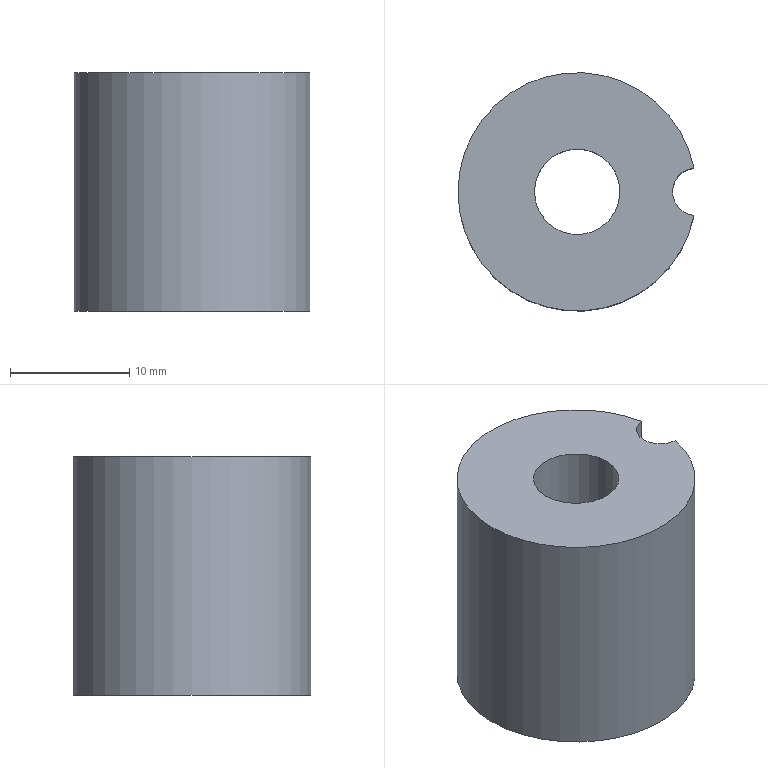Part | NX | features solid 2 | 1 solid | 7 faces | box 19.8 x 20 x 20 mm | volume 4344 mm3 | cylinder 4 | plane 3 | commonest cylinder face diameters 4 x1 7.17 x1 12.6 x1 20 x1
STEP:
#1=CARTESIAN_POINT('',(-128.447,71.998,46.841));
#2=VERTEX_POINT('',#1);
#3=CARTESIAN_POINT('',(-128.447,75.978,46.841));
#4=VERTEX_POINT('',#3);
#5=CARTESIAN_POINT('',(-128.247,73.988,46.841));
#6=DIRECTION('',(0.,0.,-1.));
#7=DIRECTION('',(-1.,0.,0.));
#8=AXIS2_PLACEMENT_3D('',#5,#6,#7);
#9=CIRCLE('',#8,2.);
#10=EDGE_CURVE('',#2,#4,#9,.T.);
#11=ORIENTED_EDGE('',*,*,#10,.T.);
#12=CARTESIAN_POINT('',(-138.247,73.988,46.841));
#13=DIRECTION('',(0.,0.,-1.));
#14=DIRECTION('',(-1.,0.,0.));
#15=AXIS2_PLACEMENT_3D('',#12,#13,#14);
#16=CIRCLE('',#15,10.);
#17=EDGE_CURVE('',#2,#4,#16,.T.);
#18=ORIENTED_EDGE('',*,*,#17,.F.);
#19=EDGE_LOOP('',(#11,#18));
#20=FACE_BOUND('',#19,.T.);
#21=CARTESIAN_POINT('',(-141.832,73.988,46.841));
#22=VERTEX_POINT('',#21);
#23=CARTESIAN_POINT('',(-138.247,73.988,46.841));
#24=DIRECTION('',(0.,0.,-1.));
#25=DIRECTION('',(-1.,0.,0.));
#26=AXIS2_PLACEMENT_3D('',#23,#24,#25);
#27=CIRCLE('',#26,3.585);
#28=EDGE_CURVE('',#22,#22,#27,.T.);
#29=ORIENTED_EDGE('',*,*,#28,.T.);
#30=EDGE_LOOP('',(#29));
#31=FACE_BOUND('',#30,.T.);
#32=CARTESIAN_POINT('',(-138.247,73.988,46.841));
#33=DIRECTION('',(0.,0.,1.));
#34=DIRECTION('',(1.,0.,0.));
#35=AXIS2_PLACEMENT_3D('',#32,#33,#34);
#36=PLANE('',#35);
#37=ADVANCED_FACE('',(#20,#31),#36,.T.);
#38=CARTESIAN_POINT('',(-128.447,75.978,26.841));
#39=VERTEX_POINT('',#38);
#40=CARTESIAN_POINT('',(-128.447,71.998,26.841));
#41=VERTEX_POINT('',#40);
#42=CARTESIAN_POINT('',(-128.247,73.988,26.841));
#43=DIRECTION('',(0.,0.,1.));
#44=DIRECTION('',(1.,0.,0.));
#45=AXIS2_PLACEMENT_3D('',#42,#43,#44);
#46=CIRCLE('',#45,2.);
#47=EDGE_CURVE('',#39,#41,#46,.T.);
#48=ORIENTED_EDGE('',*,*,#47,.T.);
#49=CARTESIAN_POINT('',(-138.247,73.988,26.841));
#50=DIRECTION('',(0.,0.,1.));
#51=DIRECTION('',(1.,0.,0.));
#52=AXIS2_PLACEMENT_3D('',#49,#50,#51);
#53=CIRCLE('',#52,10.);
#54=EDGE_CURVE('',#39,#41,#53,.T.);
#55=ORIENTED_EDGE('',*,*,#54,.F.);
#56=EDGE_LOOP('',(#48,#55));
#57=FACE_BOUND('',#56,.T.);
#58=CARTESIAN_POINT('',(-131.947,73.988,26.841));
#59=VERTEX_POINT('',#58);
#60=CARTESIAN_POINT('',(-138.247,73.988,26.841));
#61=DIRECTION('',(0.,0.,1.));
#62=DIRECTION('',(1.,0.,0.));
#63=AXIS2_PLACEMENT_3D('',#60,#61,#62);
#64=CIRCLE('',#63,6.3);
#65=EDGE_CURVE('',#59,#59,#64,.T.);
#66=ORIENTED_EDGE('',*,*,#65,.T.);
#67=EDGE_LOOP('',(#66));
#68=FACE_BOUND('',#67,.T.);
#69=CARTESIAN_POINT('',(-138.247,73.988,26.841));
#70=DIRECTION('',(0.,0.,-1.));
#71=DIRECTION('',(-1.,0.,0.));
#72=AXIS2_PLACEMENT_3D('',#69,#70,#71);
#73=PLANE('',#72);
#74=ADVANCED_FACE('',(#57,#68),#73,.T.);
#75=CARTESIAN_POINT('',(-128.447,75.978,36.841));
#76=DIRECTION('',(0.,0.,1.));
#77=VECTOR('',#76,1000.);
#78=LINE('',#75,#77);
#79=EDGE_CURVE('',#39,#4,#78,.T.);
#80=ORIENTED_EDGE('',*,*,#79,.F.);
#81=ORIENTED_EDGE('',*,*,#54,.T.);
#82=CARTESIAN_POINT('',(-128.447,71.998,36.841));
#83=DIRECTION('',(0.,0.,1.));
#84=VECTOR('',#83,1000.);
#85=LINE('',#82,#84);
#86=EDGE_CURVE('',#2,#41,#85,.F.);
#87=ORIENTED_EDGE('',*,*,#86,.F.);
#88=ORIENTED_EDGE('',*,*,#17,.T.);
#89=EDGE_LOOP('',(#80,#81,#87,#88));
#90=FACE_BOUND('',#89,.T.);
#91=CARTESIAN_POINT('',(-138.247,73.988,26.841));
#92=DIRECTION('',(0.,0.,1.));
#93=DIRECTION('',(1.,0.,0.));
#94=AXIS2_PLACEMENT_3D('',#91,#92,#93);
#95=CYLINDRICAL_SURFACE('',#94,10.);
#96=ADVANCED_FACE('',(#90),#95,.T.);
#97=CARTESIAN_POINT('',(-134.662,73.988,38.841));
#98=VERTEX_POINT('',#97);
#99=CARTESIAN_POINT('',(-138.247,73.988,38.841));
#100=DIRECTION('',(0.,0.,1.));
#101=DIRECTION('',(1.,0.,0.));
#102=AXIS2_PLACEMENT_3D('',#99,#100,#101);
#103=CIRCLE('',#102,3.585);
#104=EDGE_CURVE('',#98,#98,#103,.T.);
#105=ORIENTED_EDGE('',*,*,#104,.T.);
#106=EDGE_LOOP('',(#105));
#107=FACE_BOUND('',#106,.T.);
#108=CARTESIAN_POINT('',(-144.547,73.988,38.841));
#109=VERTEX_POINT('',#108);
#110=CARTESIAN_POINT('',(-138.247,73.988,38.841));
#111=DIRECTION('',(0.,0.,-1.));
#112=DIRECTION('',(-1.,0.,0.));
#113=AXIS2_PLACEMENT_3D('',#110,#111,#112);
#114=CIRCLE('',#113,6.3);
#115=EDGE_CURVE('',#109,#109,#114,.T.);
#116=ORIENTED_EDGE('',*,*,#115,.T.);
#117=EDGE_LOOP('',(#116));
#118=FACE_BOUND('',#117,.T.);
#119=CARTESIAN_POINT('',(-138.247,73.988,38.841));
#120=DIRECTION('',(0.,0.,1.));
#121=DIRECTION('',(1.,0.,0.));
#122=AXIS2_PLACEMENT_3D('',#119,#120,#121);
#123=PLANE('',#122);
#124=ADVANCED_FACE('',(#107,#118),#123,.F.);
#125=ORIENTED_EDGE('',*,*,#115,.F.);
#126=EDGE_LOOP('',(#125));
#127=FACE_BOUND('',#126,.T.);
#128=ORIENTED_EDGE('',*,*,#65,.F.);
#129=EDGE_LOOP('',(#128));
#130=FACE_BOUND('',#129,.T.);
#131=CARTESIAN_POINT('',(-138.247,73.988,26.841));
#132=DIRECTION('',(0.,0.,1.));
#133=DIRECTION('',(1.,0.,0.));
#134=AXIS2_PLACEMENT_3D('',#131,#132,#133);
#135=CYLINDRICAL_SURFACE('',#134,6.3);
#136=ADVANCED_FACE('',(#127,#130),#135,.F.);
#137=ORIENTED_EDGE('',*,*,#28,.F.);
#138=EDGE_LOOP('',(#137));
#139=FACE_BOUND('',#138,.T.);
#140=ORIENTED_EDGE('',*,*,#104,.F.);
#141=EDGE_LOOP('',(#140));
#142=FACE_BOUND('',#141,.T.);
#143=CARTESIAN_POINT('',(-138.247,73.988,38.841));
#144=DIRECTION('',(0.,0.,1.));
#145=DIRECTION('',(1.,0.,0.));
#146=AXIS2_PLACEMENT_3D('',#143,#144,#145);
#147=CYLINDRICAL_SURFACE('',#146,3.585);
#148=ADVANCED_FACE('',(#139,#142),#147,.F.);
#149=ORIENTED_EDGE('',*,*,#79,.T.);
#150=ORIENTED_EDGE('',*,*,#10,.F.);
#151=ORIENTED_EDGE('',*,*,#86,.T.);
#152=ORIENTED_EDGE('',*,*,#47,.F.);
#153=EDGE_LOOP('',(#149,#150,#151,#152));
#154=FACE_BOUND('',#153,.T.);
#155=CARTESIAN_POINT('',(-128.247,73.988,26.841));
#156=DIRECTION('',(0.,0.,1.));
#157=DIRECTION('',(1.,0.,0.));
#158=AXIS2_PLACEMENT_3D('',#155,#156,#157);
#159=CYLINDRICAL_SURFACE('',#158,2.);
#160=ADVANCED_FACE('',(#154),#159,.F.);
#161=CLOSED_SHELL('',(#37,#74,#96,#124,#136,#148,#160));
#162=MANIFOLD_SOLID_BREP('',#161);
#163=(LENGTH_UNIT()NAMED_UNIT(*)SI_UNIT(.MILLI.,.METRE.));
#164=UNCERTAINTY_MEASURE_WITH_UNIT(LENGTH_MEASURE(0.00001),#163,'','');
#165=(NAMED_UNIT(*)PLANE_ANGLE_UNIT()SI_UNIT($,.RADIAN.));
#166=(NAMED_UNIT(*)SI_UNIT($,.STERADIAN.)SOLID_ANGLE_UNIT());
#167=(GEOMETRIC_REPRESENTATION_CONTEXT(3)GLOBAL_UNCERTAINTY_ASSIGNED_CONTEXT((#164))GLOBAL_UNIT_ASSIGNED_CONTEXT((#163,#165,#166))REPRESENTATION_CONTEXT('',''));
#168=ADVANCED_BREP_SHAPE_REPRESENTATION('',(#162),#167);